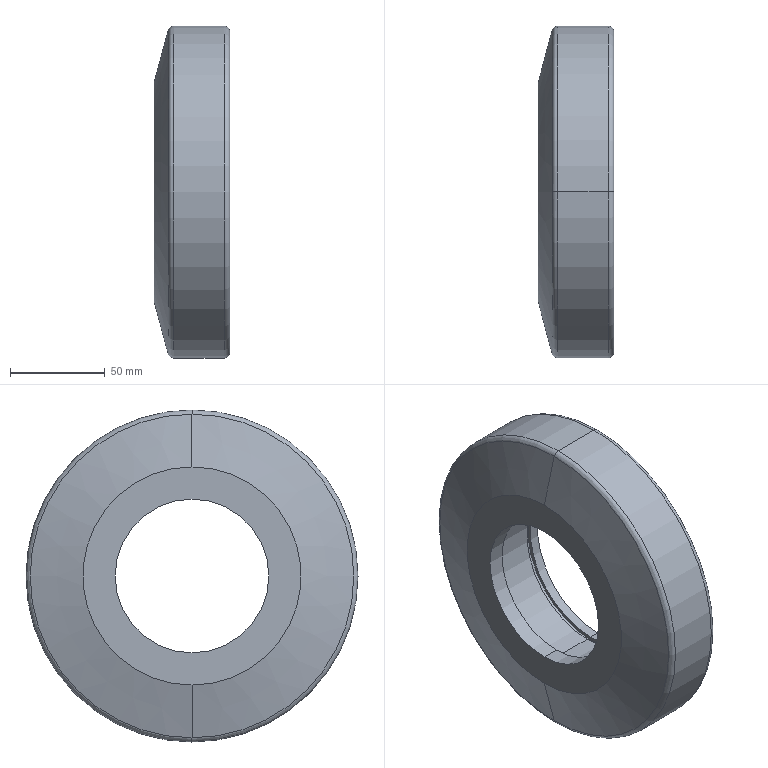Part | STEP file | 02-Guide roller 2 | 1 solid | 21 faces | box 40 x 175 x 175 mm | volume 657116 mm3 | cylinder 10 | plane 5 | torus 4 | cone 2 | commonest cylinder face diameters 90 x4 81 x2 93.5 x2 175 x2
STEP:
#1=CARTESIAN_POINT('',(0.,0.,0.));
#2=DIRECTION('',(0.,0.,1.));
#3=DIRECTION('',(1.,0.,0.));
#4=AXIS2_PLACEMENT_3D('',#1,#2,#3);
#5=CARTESIAN_POINT('',(9.,0.,40.5));
#6=VERTEX_POINT('',#5);
#7=CARTESIAN_POINT('',(0.,0.,40.5));
#8=VERTEX_POINT('',#7);
#9=CARTESIAN_POINT('',(0.,0.,40.5));
#10=DIRECTION('',(-1.,0.,0.));
#11=VECTOR('',#10,1.);
#12=LINE('',#9,#11);
#13=CARTESIAN_POINT('',(0.,0.,0.));
#14=DIRECTION('',(-1.,0.,0.));
#15=DIRECTION('',(0.,0.,1.));
#16=AXIS2_PLACEMENT_3D('',#13,#14,#15);
#17=CYLINDRICAL_SURFACE('',#16,40.5);
#18=CARTESIAN_POINT('',(6.283,0.));
#19=DIRECTION('',(0.,1.));
#20=VECTOR('',#19,1.);
#21=LINE('',#18,#20);
#22=(GEOMETRIC_REPRESENTATION_CONTEXT(2)PARAMETRIC_REPRESENTATION_CONTEXT()REPRESENTATION_CONTEXT('',''));
#23=DEFINITIONAL_REPRESENTATION('',(#21),#22);
#24=PCURVE('',#17,#23);
#25=CARTESIAN_POINT('',(0.,0.,0.));
#26=DIRECTION('',(-1.,0.,0.));
#27=DIRECTION('',(0.,0.,1.));
#28=AXIS2_PLACEMENT_3D('',#25,#26,#27);
#29=CYLINDRICAL_SURFACE('',#28,40.5);
#30=CARTESIAN_POINT('',(0.,0.));
#31=DIRECTION('',(0.,1.));
#32=VECTOR('',#31,1.);
#33=LINE('',#30,#32);
#34=(GEOMETRIC_REPRESENTATION_CONTEXT(2)PARAMETRIC_REPRESENTATION_CONTEXT()REPRESENTATION_CONTEXT('',''));
#35=DEFINITIONAL_REPRESENTATION('',(#33),#34);
#36=PCURVE('',#29,#35);
#37=SURFACE_CURVE('',#12,(#24,#36),.PCURVE_S1.);
#38=EDGE_CURVE('',#6,#8,#37,.T.);
#39=ORIENTED_EDGE('',*,*,#38,.T.);
#40=CARTESIAN_POINT('',(0.,0.,-40.5));
#41=VERTEX_POINT('',#40);
#42=CARTESIAN_POINT('',(0.,0.,0.));
#43=DIRECTION('',(-1.,0.,0.));
#44=DIRECTION('',(0.,0.,1.));
#45=AXIS2_PLACEMENT_3D('',#42,#43,#44);
#46=CIRCLE('',#45,40.5);
#47=CARTESIAN_POINT('',(0.,0.));
#48=DIRECTION('',(1.,0.));
#49=VECTOR('',#48,1.);
#50=LINE('',#47,#49);
#51=(GEOMETRIC_REPRESENTATION_CONTEXT(2)PARAMETRIC_REPRESENTATION_CONTEXT()REPRESENTATION_CONTEXT('',''));
#52=DEFINITIONAL_REPRESENTATION('',(#50),#51);
#53=PCURVE('',#17,#52);
#54=CARTESIAN_POINT('',(0.,40.5,0.));
#55=DIRECTION('',(1.,0.,0.));
#56=DIRECTION('',(0.,0.,-1.));
#57=AXIS2_PLACEMENT_3D('',#54,#55,#56);
#58=PLANE('',#57);
#59=CARTESIAN_POINT('',(-40.5,-40.5));
#60=CARTESIAN_POINT('',(-40.5,29.648));
#61=CARTESIAN_POINT('',(20.25,-5.426));
#62=CARTESIAN_POINT('',(81.,-40.5));
#63=CARTESIAN_POINT('',(20.25,-75.574));
#64=CARTESIAN_POINT('',(-40.5,-110.648));
#65=CARTESIAN_POINT('',(-40.5,-40.5));
#66=(BOUNDED_CURVE()B_SPLINE_CURVE(2,(#59,#60,#61,#62,#63,#64,#65),.UNSPECIFIED.,.T.,.F.)B_SPLINE_CURVE_WITH_KNOTS((1,2,2,2,2,1),(-2.094,0.,2.094,4.189,6.283,8.378),.UNSPECIFIED.)CURVE()GEOMETRIC_REPRESENTATION_ITEM()RATIONAL_B_SPLINE_CURVE((1.,0.5,1.,0.5,1.,0.5,1.))REPRESENTATION_ITEM(''));
#67=(GEOMETRIC_REPRESENTATION_CONTEXT(2)PARAMETRIC_REPRESENTATION_CONTEXT()REPRESENTATION_CONTEXT('',''));
#68=DEFINITIONAL_REPRESENTATION('',(#66),#67);
#69=PCURVE('',#58,#68);
#70=SURFACE_CURVE('',#46,(#53,#69),.PCURVE_S1.);
#71=EDGE_CURVE('',#41,#8,#70,.T.);
#72=ORIENTED_EDGE('',*,*,#71,.F.);
#73=CARTESIAN_POINT('',(9.,0.,-40.5));
#74=VERTEX_POINT('',#73);
#75=CARTESIAN_POINT('',(0.,0.,-40.5));
#76=DIRECTION('',(-1.,0.,0.));
#77=VECTOR('',#76,1.);
#78=LINE('',#75,#77);
#79=CARTESIAN_POINT('',(3.142,0.));
#80=DIRECTION('',(0.,1.));
#81=VECTOR('',#80,1.);
#82=LINE('',#79,#81);
#83=(GEOMETRIC_REPRESENTATION_CONTEXT(2)PARAMETRIC_REPRESENTATION_CONTEXT()REPRESENTATION_CONTEXT('',''));
#84=DEFINITIONAL_REPRESENTATION('',(#82),#83);
#85=PCURVE('',#17,#84);
#86=CARTESIAN_POINT('',(3.142,0.));
#87=DIRECTION('',(0.,1.));
#88=VECTOR('',#87,1.);
#89=LINE('',#86,#88);
#90=(GEOMETRIC_REPRESENTATION_CONTEXT(2)PARAMETRIC_REPRESENTATION_CONTEXT()REPRESENTATION_CONTEXT('',''));
#91=DEFINITIONAL_REPRESENTATION('',(#89),#90);
#92=PCURVE('',#29,#91);
#93=SURFACE_CURVE('',#78,(#85,#92),.PCURVE_S1.);
#94=EDGE_CURVE('',#74,#41,#93,.T.);
#95=ORIENTED_EDGE('',*,*,#94,.F.);
#96=CARTESIAN_POINT('',(9.,0.,0.));
#97=DIRECTION('',(-1.,0.,0.));
#98=DIRECTION('',(0.,0.,1.));
#99=AXIS2_PLACEMENT_3D('',#96,#97,#98);
#100=CIRCLE('',#99,40.5);
#101=CARTESIAN_POINT('',(0.,-9.));
#102=DIRECTION('',(1.,0.));
#103=VECTOR('',#102,1.);
#104=LINE('',#101,#103);
#105=(GEOMETRIC_REPRESENTATION_CONTEXT(2)PARAMETRIC_REPRESENTATION_CONTEXT()REPRESENTATION_CONTEXT('',''));
#106=DEFINITIONAL_REPRESENTATION('',(#104),#105);
#107=PCURVE('',#17,#106);
#108=CARTESIAN_POINT('',(9.,45.,0.));
#109=DIRECTION('',(-1.,0.,0.));
#110=DIRECTION('',(0.,0.,1.));
#111=AXIS2_PLACEMENT_3D('',#108,#109,#110);
#112=PLANE('',#111);
#113=CARTESIAN_POINT('',(0.,-45.));
#114=DIRECTION('',(1.,0.));
#115=AXIS2_PLACEMENT_2D('',#113,#114);
#116=CIRCLE('',#115,40.5);
#117=(GEOMETRIC_REPRESENTATION_CONTEXT(2)PARAMETRIC_REPRESENTATION_CONTEXT()REPRESENTATION_CONTEXT('',''));
#118=DEFINITIONAL_REPRESENTATION('',(#116),#117);
#119=PCURVE('',#112,#118);
#120=SURFACE_CURVE('',#100,(#107,#119),.PCURVE_S1.);
#121=EDGE_CURVE('',#74,#6,#120,.T.);
#122=ORIENTED_EDGE('',*,*,#121,.T.);
#123=EDGE_LOOP('',(#39,#72,#95,#122));
#124=FACE_BOUND('',#123,.F.);
#125=ADVANCED_FACE('',(#124),#17,.F.);
#126=CARTESIAN_POINT('',(32.,0.,45.));
#127=VERTEX_POINT('',#126);
#128=CARTESIAN_POINT('',(9.,0.,45.));
#129=VERTEX_POINT('',#128);
#130=CARTESIAN_POINT('',(0.,0.,45.));
#131=DIRECTION('',(-1.,0.,0.));
#132=VECTOR('',#131,1.);
#133=LINE('',#130,#132);
#134=CARTESIAN_POINT('',(0.,0.,0.));
#135=DIRECTION('',(-1.,0.,0.));
#136=DIRECTION('',(0.,0.,1.));
#137=AXIS2_PLACEMENT_3D('',#134,#135,#136);
#138=CYLINDRICAL_SURFACE('',#137,45.);
#139=CARTESIAN_POINT('',(6.283,0.));
#140=DIRECTION('',(0.,1.));
#141=VECTOR('',#140,1.);
#142=LINE('',#139,#141);
#143=(GEOMETRIC_REPRESENTATION_CONTEXT(2)PARAMETRIC_REPRESENTATION_CONTEXT()REPRESENTATION_CONTEXT('',''));
#144=DEFINITIONAL_REPRESENTATION('',(#142),#143);
#145=PCURVE('',#138,#144);
#146=CARTESIAN_POINT('',(0.,0.,0.));
#147=DIRECTION('',(-1.,0.,0.));
#148=DIRECTION('',(0.,0.,1.));
#149=AXIS2_PLACEMENT_3D('',#146,#147,#148);
#150=CYLINDRICAL_SURFACE('',#149,45.);
#151=CARTESIAN_POINT('',(0.,0.));
#152=DIRECTION('',(0.,1.));
#153=VECTOR('',#152,1.);
#154=LINE('',#151,#153);
#155=(GEOMETRIC_REPRESENTATION_CONTEXT(2)PARAMETRIC_REPRESENTATION_CONTEXT()REPRESENTATION_CONTEXT('',''));
#156=DEFINITIONAL_REPRESENTATION('',(#154),#155);
#157=PCURVE('',#150,#156);
#158=SURFACE_CURVE('',#133,(#145,#157),.PCURVE_S1.);
#159=EDGE_CURVE('',#127,#129,#158,.T.);
#160=ORIENTED_EDGE('',*,*,#159,.T.);
#161=CARTESIAN_POINT('',(9.,0.,-45.));
#162=VERTEX_POINT('',#161);
#163=CARTESIAN_POINT('',(9.,0.,0.));
#164=DIRECTION('',(-1.,0.,0.));
#165=DIRECTION('',(0.,0.,1.));
#166=AXIS2_PLACEMENT_3D('',#163,#164,#165);
#167=CIRCLE('',#166,45.);
#168=CARTESIAN_POINT('',(0.,-9.));
#169=DIRECTION('',(1.,0.));
#170=VECTOR('',#169,1.);
#171=LINE('',#168,#170);
#172=(GEOMETRIC_REPRESENTATION_CONTEXT(2)PARAMETRIC_REPRESENTATION_CONTEXT()REPRESENTATION_CONTEXT('',''));
#173=DEFINITIONAL_REPRESENTATION('',(#171),#172);
#174=PCURVE('',#138,#173);
#175=CARTESIAN_POINT('',(0.,-45.));
#176=DIRECTION('',(1.,0.));
#177=AXIS2_PLACEMENT_2D('',#175,#176);
#178=CIRCLE('',#177,45.);
#179=(GEOMETRIC_REPRESENTATION_CONTEXT(2)PARAMETRIC_REPRESENTATION_CONTEXT()REPRESENTATION_CONTEXT('',''));
#180=DEFINITIONAL_REPRESENTATION('',(#178),#179);
#181=PCURVE('',#112,#180);
#182=SURFACE_CURVE('',#167,(#174,#181),.PCURVE_S1.);
#183=EDGE_CURVE('',#162,#129,#182,.T.);
#184=ORIENTED_EDGE('',*,*,#183,.F.);
#185=CARTESIAN_POINT('',(32.,0.,-45.));
#186=VERTEX_POINT('',#185);
#187=CARTESIAN_POINT('',(0.,0.,-45.));
#188=DIRECTION('',(-1.,0.,0.));
#189=VECTOR('',#188,1.);
#190=LINE('',#187,#189);
#191=CARTESIAN_POINT('',(3.142,0.));
#192=DIRECTION('',(0.,1.));
#193=VECTOR('',#192,1.);
#194=LINE('',#191,#193);
#195=(GEOMETRIC_REPRESENTATION_CONTEXT(2)PARAMETRIC_REPRESENTATION_CONTEXT()REPRESENTATION_CONTEXT('',''));
#196=DEFINITIONAL_REPRESENTATION('',(#194),#195);
#197=PCURVE('',#138,#196);
#198=CARTESIAN_POINT('',(3.142,0.));
#199=DIRECTION('',(0.,1.));
#200=VECTOR('',#199,1.);
#201=LINE('',#198,#200);
#202=(GEOMETRIC_REPRESENTATION_CONTEXT(2)PARAMETRIC_REPRESENTATION_CONTEXT()REPRESENTATION_CONTEXT('',''));
#203=DEFINITIONAL_REPRESENTATION('',(#201),#202);
#204=PCURVE('',#150,#203);
#205=SURFACE_CURVE('',#190,(#197,#204),.PCURVE_S1.);
#206=EDGE_CURVE('',#186,#162,#205,.T.);
#207=ORIENTED_EDGE('',*,*,#206,.F.);
#208=CARTESIAN_POINT('',(32.,0.,0.));
#209=DIRECTION('',(-1.,0.,0.));
#210=DIRECTION('',(0.,0.,1.));
#211=AXIS2_PLACEMENT_3D('',#208,#209,#210);
#212=CIRCLE('',#211,45.);
#213=CARTESIAN_POINT('',(0.,-32.));
#214=DIRECTION('',(1.,0.));
#215=VECTOR('',#214,1.);
#216=LINE('',#213,#215);
#217=(GEOMETRIC_REPRESENTATION_CONTEXT(2)PARAMETRIC_REPRESENTATION_CONTEXT()REPRESENTATION_CONTEXT('',''));
#218=DEFINITIONAL_REPRESENTATION('',(#216),#217);
#219=PCURVE('',#138,#218);
#220=CARTESIAN_POINT('',(32.,46.75,0.));
#221=DIRECTION('',(-1.,0.,0.));
#222=DIRECTION('',(0.,0.,1.));
#223=AXIS2_PLACEMENT_3D('',#220,#221,#222);
#224=PLANE('',#223);
#225=CARTESIAN_POINT('',(0.,-46.75));
#226=DIRECTION('',(1.,0.));
#227=AXIS2_PLACEMENT_2D('',#225,#226);
#228=CIRCLE('',#227,45.);
#229=(GEOMETRIC_REPRESENTATION_CONTEXT(2)PARAMETRIC_REPRESENTATION_CONTEXT()REPRESENTATION_CONTEXT('',''));
#230=DEFINITIONAL_REPRESENTATION('',(#228),#229);
#231=PCURVE('',#224,#230);
#232=SURFACE_CURVE('',#212,(#219,#231),.PCURVE_S1.);
#233=EDGE_CURVE('',#186,#127,#232,.T.);
#234=ORIENTED_EDGE('',*,*,#233,.T.);
#235=EDGE_LOOP('',(#160,#184,#207,#234));
#236=FACE_BOUND('',#235,.F.);
#237=ADVANCED_FACE('',(#236),#138,.F.);
#238=CARTESIAN_POINT('',(34.7,0.,46.75));
#239=VERTEX_POINT('',#238);
#240=CARTESIAN_POINT('',(32.,0.,46.75));
#241=VERTEX_POINT('',#240);
#242=CARTESIAN_POINT('',(0.,0.,46.75));
#243=DIRECTION('',(-1.,0.,0.));
#244=VECTOR('',#243,1.);
#245=LINE('',#242,#244);
#246=CARTESIAN_POINT('',(0.,0.,0.));
#247=DIRECTION('',(-1.,0.,0.));
#248=DIRECTION('',(0.,0.,1.));
#249=AXIS2_PLACEMENT_3D('',#246,#247,#248);
#250=CYLINDRICAL_SURFACE('',#249,46.75);
#251=CARTESIAN_POINT('',(6.283,0.));
#252=DIRECTION('',(0.,1.));
#253=VECTOR('',#252,1.);
#254=LINE('',#251,#253);
#255=(GEOMETRIC_REPRESENTATION_CONTEXT(2)PARAMETRIC_REPRESENTATION_CONTEXT()REPRESENTATION_CONTEXT('',''));
#256=DEFINITIONAL_REPRESENTATION('',(#254),#255);
#257=PCURVE('',#250,#256);
#258=CARTESIAN_POINT('',(0.,0.,0.));
#259=DIRECTION('',(-1.,0.,0.));
#260=DIRECTION('',(0.,0.,1.));
#261=AXIS2_PLACEMENT_3D('',#258,#259,#260);
#262=CYLINDRICAL_SURFACE('',#261,46.75);
#263=CARTESIAN_POINT('',(0.,0.));
#264=DIRECTION('',(0.,1.));
#265=VECTOR('',#264,1.);
#266=LINE('',#263,#265);
#267=(GEOMETRIC_REPRESENTATION_CONTEXT(2)PARAMETRIC_REPRESENTATION_CONTEXT()REPRESENTATION_CONTEXT('',''));
#268=DEFINITIONAL_REPRESENTATION('',(#266),#267);
#269=PCURVE('',#262,#268);
#270=SURFACE_CURVE('',#245,(#257,#269),.PCURVE_S1.);
#271=EDGE_CURVE('',#239,#241,#270,.T.);
#272=ORIENTED_EDGE('',*,*,#271,.T.);
#273=CARTESIAN_POINT('',(32.,0.,-46.75));
#274=VERTEX_POINT('',#273);
#275=CARTESIAN_POINT('',(32.,0.,0.));
#276=DIRECTION('',(-1.,0.,0.));
#277=DIRECTION('',(0.,0.,1.));
#278=AXIS2_PLACEMENT_3D('',#275,#276,#277);
#279=CIRCLE('',#278,46.75);
#280=CARTESIAN_POINT('',(0.,-32.));
#281=DIRECTION('',(1.,0.));
#282=VECTOR('',#281,1.);
#283=LINE('',#280,#282);
#284=(GEOMETRIC_REPRESENTATION_CONTEXT(2)PARAMETRIC_REPRESENTATION_CONTEXT()REPRESENTATION_CONTEXT('',''));
#285=DEFINITIONAL_REPRESENTATION('',(#283),#284);
#286=PCURVE('',#250,#285);
#287=CARTESIAN_POINT('',(0.,-46.75));
#288=DIRECTION('',(1.,0.));
#289=AXIS2_PLACEMENT_2D('',#287,#288);
#290=CIRCLE('',#289,46.75);
#291=(GEOMETRIC_REPRESENTATION_CONTEXT(2)PARAMETRIC_REPRESENTATION_CONTEXT()REPRESENTATION_CONTEXT('',''));
#292=DEFINITIONAL_REPRESENTATION('',(#290),#291);
#293=PCURVE('',#224,#292);
#294=SURFACE_CURVE('',#279,(#286,#293),.PCURVE_S1.);
#295=EDGE_CURVE('',#274,#241,#294,.T.);
#296=ORIENTED_EDGE('',*,*,#295,.F.);
#297=CARTESIAN_POINT('',(34.7,0.,-46.75));
#298=VERTEX_POINT('',#297);
#299=CARTESIAN_POINT('',(0.,0.,-46.75));
#300=DIRECTION('',(-1.,0.,0.));
#301=VECTOR('',#300,1.);
#302=LINE('',#299,#301);
#303=CARTESIAN_POINT('',(3.142,0.));
#304=DIRECTION('',(0.,1.));
#305=VECTOR('',#304,1.);
#306=LINE('',#303,#305);
#307=(GEOMETRIC_REPRESENTATION_CONTEXT(2)PARAMETRIC_REPRESENTATION_CONTEXT()REPRESENTATION_CONTEXT('',''));
#308=DEFINITIONAL_REPRESENTATION('',(#306),#307);
#309=PCURVE('',#250,#308);
#310=CARTESIAN_POINT('',(3.142,0.));
#311=DIRECTION('',(0.,1.));
#312=VECTOR('',#311,1.);
#313=LINE('',#310,#312);
#314=(GEOMETRIC_REPRESENTATION_CONTEXT(2)PARAMETRIC_REPRESENTATION_CONTEXT()REPRESENTATION_CONTEXT('',''));
#315=DEFINITIONAL_REPRESENTATION('',(#313),#314);
#316=PCURVE('',#262,#315);
#317=SURFACE_CURVE('',#302,(#309,#316),.PCURVE_S1.);
#318=EDGE_CURVE('',#298,#274,#317,.T.);
#319=ORIENTED_EDGE('',*,*,#318,.F.);
#320=CARTESIAN_POINT('',(34.7,0.,0.));
#321=DIRECTION('',(-1.,0.,0.));
#322=DIRECTION('',(0.,0.,1.));
#323=AXIS2_PLACEMENT_3D('',#320,#321,#322);
#324=CIRCLE('',#323,46.75);
#325=CARTESIAN_POINT('',(0.,-34.7));
#326=DIRECTION('',(1.,0.));
#327=VECTOR('',#326,1.);
#328=LINE('',#325,#327);
#329=(GEOMETRIC_REPRESENTATION_CONTEXT(2)PARAMETRIC_REPRESENTATION_CONTEXT()REPRESENTATION_CONTEXT('',''));
#330=DEFINITIONAL_REPRESENTATION('',(#328),#329);
#331=PCURVE('',#250,#330);
#332=CARTESIAN_POINT('',(34.7,45.,0.));
#333=DIRECTION('',(1.,0.,0.));
#334=DIRECTION('',(0.,0.,-1.));
#335=AXIS2_PLACEMENT_3D('',#332,#333,#334);
#336=PLANE('',#335);
#337=CARTESIAN_POINT('',(-46.75,-45.));
#338=CARTESIAN_POINT('',(-46.75,35.973));
#339=CARTESIAN_POINT('',(23.375,-4.513));
#340=CARTESIAN_POINT('',(93.5,-45.));
#341=CARTESIAN_POINT('',(23.375,-85.487));
#342=CARTESIAN_POINT('',(-46.75,-125.973));
#343=CARTESIAN_POINT('',(-46.75,-45.));
#344=(BOUNDED_CURVE()B_SPLINE_CURVE(2,(#337,#338,#339,#340,#341,#342,#343),.UNSPECIFIED.,.T.,.F.)B_SPLINE_CURVE_WITH_KNOTS((1,2,2,2,2,1),(-2.094,0.,2.094,4.189,6.283,8.378),.UNSPECIFIED.)CURVE()GEOMETRIC_REPRESENTATION_ITEM()RATIONAL_B_SPLINE_CURVE((1.,0.5,1.,0.5,1.,0.5,1.))REPRESENTATION_ITEM(''));
#345=(GEOMETRIC_REPRESENTATION_CONTEXT(2)PARAMETRIC_REPRESENTATION_CONTEXT()REPRESENTATION_CONTEXT('',''));
#346=DEFINITIONAL_REPRESENTATION('',(#344),#345);
#347=PCURVE('',#336,#346);
#348=SURFACE_CURVE('',#324,(#331,#347),.PCURVE_S1.);
#349=EDGE_CURVE('',#298,#239,#348,.T.);
#350=ORIENTED_EDGE('',*,*,#349,.T.);
#351=EDGE_LOOP('',(#272,#296,#319,#350));
#352=FACE_BOUND('',#351,.F.);
#353=ADVANCED_FACE('',(#352),#250,.F.);
#354=CARTESIAN_POINT('',(40.,0.,45.));
#355=VERTEX_POINT('',#354);
#356=CARTESIAN_POINT('',(34.7,0.,45.));
#357=VERTEX_POINT('',#356);
#358=CARTESIAN_POINT('',(0.,0.,45.));
#359=DIRECTION('',(-1.,0.,0.));
#360=VECTOR('',#359,1.);
#361=LINE('',#358,#360);
#362=CARTESIAN_POINT('',(0.,0.,0.));
#363=DIRECTION('',(-1.,0.,0.));
#364=DIRECTION('',(0.,0.,1.));
#365=AXIS2_PLACEMENT_3D('',#362,#363,#364);
#366=CYLINDRICAL_SURFACE('',#365,45.);
#367=CARTESIAN_POINT('',(6.283,0.));
#368=DIRECTION('',(0.,1.));
#369=VECTOR('',#368,1.);
#370=LINE('',#367,#369);
#371=(GEOMETRIC_REPRESENTATION_CONTEXT(2)PARAMETRIC_REPRESENTATION_CONTEXT()REPRESENTATION_CONTEXT('',''));
#372=DEFINITIONAL_REPRESENTATION('',(#370),#371);
#373=PCURVE('',#366,#372);
#374=CARTESIAN_POINT('',(0.,0.,0.));
#375=DIRECTION('',(-1.,0.,0.));
#376=DIRECTION('',(0.,0.,1.));
#377=AXIS2_PLACEMENT_3D('',#374,#375,#376);
#378=CYLINDRICAL_SURFACE('',#377,45.);
#379=CARTESIAN_POINT('',(0.,0.));
#380=DIRECTION('',(0.,1.));
#381=VECTOR('',#380,1.);
#382=LINE('',#379,#381);
#383=(GEOMETRIC_REPRESENTATION_CONTEXT(2)PARAMETRIC_REPRESENTATION_CONTEXT()REPRESENTATION_CONTEXT('',''));
#384=DEFINITIONAL_REPRESENTATION('',(#382),#383);
#385=PCURVE('',#378,#384);
#386=SURFACE_CURVE('',#361,(#373,#385),.PCURVE_S1.);
#387=EDGE_CURVE('',#355,#357,#386,.T.);
#388=ORIENTED_EDGE('',*,*,#387,.T.);
#389=CARTESIAN_POINT('',(34.7,0.,-45.));
#390=VERTEX_POINT('',#389);
#391=CARTESIAN_POINT('',(34.7,0.,0.));
#392=DIRECTION('',(-1.,0.,0.));
#393=DIRECTION('',(0.,0.,1.));
#394=AXIS2_PLACEMENT_3D('',#391,#392,#393);
#395=CIRCLE('',#394,45.);
#396=CARTESIAN_POINT('',(0.,-34.7));
#397=DIRECTION('',(1.,0.));
#398=VECTOR('',#397,1.);
#399=LINE('',#396,#398);
#400=(GEOMETRIC_REPRESENTATION_CONTEXT(2)PARAMETRIC_REPRESENTATION_CONTEXT()REPRESENTATION_CONTEXT('',''));
#401=DEFINITIONAL_REPRESENTATION('',(#399),#400);
#402=PCURVE('',#366,#401);
#403=CARTESIAN_POINT('',(-45.,-45.));
#404=CARTESIAN_POINT('',(-45.,32.942));
#405=CARTESIAN_POINT('',(22.5,-6.029));
#406=CARTESIAN_POINT('',(90.,-45.));
#407=CARTESIAN_POINT('',(22.5,-83.971));
#408=CARTESIAN_POINT('',(-45.,-122.942));
#409=CARTESIAN_POINT('',(-45.,-45.));
#410=(BOUNDED_CURVE()B_SPLINE_CURVE(2,(#403,#404,#405,#406,#407,#408,#409),.UNSPECIFIED.,.T.,.F.)B_SPLINE_CURVE_WITH_KNOTS((1,2,2,2,2,1),(-2.094,0.,2.094,4.189,6.283,8.378),.UNSPECIFIED.)CURVE()GEOMETRIC_REPRESENTATION_ITEM()RATIONAL_B_SPLINE_CURVE((1.,0.5,1.,0.5,1.,0.5,1.))REPRESENTATION_ITEM(''));
#411=(GEOMETRIC_REPRESENTATION_CONTEXT(2)PARAMETRIC_REPRESENTATION_CONTEXT()REPRESENTATION_CONTEXT('',''));
#412=DEFINITIONAL_REPRESENTATION('',(#410),#411);
#413=PCURVE('',#336,#412);
#414=SURFACE_CURVE('',#395,(#402,#413),.PCURVE_S1.);
#415=EDGE_CURVE('',#390,#357,#414,.T.);
#416=ORIENTED_EDGE('',*,*,#415,.F.);
#417=CARTESIAN_POINT('',(40.,0.,-45.));
#418=VERTEX_POINT('',#417);
#419=CARTESIAN_POINT('',(0.,0.,-45.));
#420=DIRECTION('',(-1.,0.,0.));
#421=VECTOR('',#420,1.);
#422=LINE('',#419,#421);
#423=CARTESIAN_POINT('',(3.142,0.));
#424=DIRECTION('',(0.,1.));
#425=VECTOR('',#424,1.);
#426=LINE('',#423,#425);
#427=(GEOMETRIC_REPRESENTATION_CONTEXT(2)PARAMETRIC_REPRESENTATION_CONTEXT()REPRESENTATION_CONTEXT('',''));
#428=DEFINITIONAL_REPRESENTATION('',(#426),#427);
#429=PCURVE('',#366,#428);
#430=CARTESIAN_POINT('',(3.142,0.));
#431=DIRECTION('',(0.,1.));
#432=VECTOR('',#431,1.);
#433=LINE('',#430,#432);
#434=(GEOMETRIC_REPRESENTATION_CONTEXT(2)PARAMETRIC_REPRESENTATION_CONTEXT()REPRESENTATION_CONTEXT('',''));
#435=DEFINITIONAL_REPRESENTATION('',(#433),#434);
#436=PCURVE('',#378,#435);
#437=SURFACE_CURVE('',#422,(#429,#436),.PCURVE_S1.);
#438=EDGE_CURVE('',#418,#390,#437,.T.);
#439=ORIENTED_EDGE('',*,*,#438,.F.);
#440=CARTESIAN_POINT('',(40.,0.,0.));
#441=DIRECTION('',(-1.,0.,0.));
#442=DIRECTION('',(0.,0.,1.));
#443=AXIS2_PLACEMENT_3D('',#440,#441,#442);
#444=CIRCLE('',#443,45.);
#445=CARTESIAN_POINT('',(0.,-40.));
#446=DIRECTION('',(1.,0.));
#447=VECTOR('',#446,1.);
#448=LINE('',#445,#447);
#449=(GEOMETRIC_REPRESENTATION_CONTEXT(2)PARAMETRIC_REPRESENTATION_CONTEXT()REPRESENTATION_CONTEXT('',''));
#450=DEFINITIONAL_REPRESENTATION('',(#448),#449);
#451=PCURVE('',#366,#450);
#452=CARTESIAN_POINT('',(40.,84.5,0.));
#453=DIRECTION('',(-1.,0.,0.));
#454=DIRECTION('',(0.,0.,1.));
#455=AXIS2_PLACEMENT_3D('',#452,#453,#454);
#456=PLANE('',#455);
#457=CARTESIAN_POINT('',(0.,-84.5));
#458=DIRECTION('',(1.,0.));
#459=AXIS2_PLACEMENT_2D('',#457,#458);
#460=CIRCLE('',#459,45.);
#461=(GEOMETRIC_REPRESENTATION_CONTEXT(2)PARAMETRIC_REPRESENTATION_CONTEXT()REPRESENTATION_CONTEXT('',''));
#462=DEFINITIONAL_REPRESENTATION('',(#460),#461);
#463=PCURVE('',#456,#462);
#464=SURFACE_CURVE('',#444,(#451,#463),.PCURVE_S1.);
#465=EDGE_CURVE('',#418,#355,#464,.T.);
#466=ORIENTED_EDGE('',*,*,#465,.T.);
#467=EDGE_LOOP('',(#388,#416,#439,#466));
#468=FACE_BOUND('',#467,.F.);
#469=ADVANCED_FACE('',(#468),#366,.F.);
#470=CARTESIAN_POINT('',(40.,0.,84.5));
#471=VERTEX_POINT('',#470);
#472=CARTESIAN_POINT('',(40.,0.,-84.5));
#473=VERTEX_POINT('',#472);
#474=CARTESIAN_POINT('',(40.,0.,0.));
#475=DIRECTION('',(-1.,0.,0.));
#476=DIRECTION('',(0.,0.,1.));
#477=AXIS2_PLACEMENT_3D('',#474,#475,#476);
#478=CIRCLE('',#477,84.5);
#479=CARTESIAN_POINT('',(37.,0.,0.));
#480=DIRECTION('',(-1.,0.,0.));
#481=DIRECTION('',(0.,0.,1.));
#482=AXIS2_PLACEMENT_3D('',#479,#480,#481);
#483=TOROIDAL_SURFACE('',#482,84.5,3.);
#484=CARTESIAN_POINT('',(0.,4.712));
#485=DIRECTION('',(1.,0.));
#486=VECTOR('',#485,1.);
#487=LINE('',#484,#486);
#488=(GEOMETRIC_REPRESENTATION_CONTEXT(2)PARAMETRIC_REPRESENTATION_CONTEXT()REPRESENTATION_CONTEXT('',''));
#489=DEFINITIONAL_REPRESENTATION('',(#487),#488);
#490=PCURVE('',#483,#489);
#491=CARTESIAN_POINT('',(0.,-84.5));
#492=DIRECTION('',(1.,0.));
#493=AXIS2_PLACEMENT_2D('',#491,#492);
#494=CIRCLE('',#493,84.5);
#495=(GEOMETRIC_REPRESENTATION_CONTEXT(2)PARAMETRIC_REPRESENTATION_CONTEXT()REPRESENTATION_CONTEXT('',''));
#496=DEFINITIONAL_REPRESENTATION('',(#494),#495);
#497=PCURVE('',#456,#496);
#498=SURFACE_CURVE('',#478,(#490,#497),.PCURVE_S1.);
#499=EDGE_CURVE('',#471,#473,#498,.T.);
#500=ORIENTED_EDGE('',*,*,#499,.T.);
#501=CARTESIAN_POINT('',(37.,0.,-87.5));
#502=VERTEX_POINT('',#501);
#503=CARTESIAN_POINT('',(37.,0.,-84.5));
#504=DIRECTION('',(0.,1.,0.));
#505=DIRECTION('',(0.,0.,1.));
#506=AXIS2_PLACEMENT_3D('',#503,#504,#505);
#507=CIRCLE('',#506,3.);
#508=CARTESIAN_POINT('',(3.142,3.142));
#509=DIRECTION('',(0.,1.));
#510=VECTOR('',#509,1.);
#511=LINE('',#508,#510);
#512=(GEOMETRIC_REPRESENTATION_CONTEXT(2)PARAMETRIC_REPRESENTATION_CONTEXT()REPRESENTATION_CONTEXT('',''));
#513=DEFINITIONAL_REPRESENTATION('',(#511),#512);
#514=PCURVE('',#483,#513);
#515=CARTESIAN_POINT('',(37.,0.,0.));
#516=DIRECTION('',(-1.,0.,0.));
#517=DIRECTION('',(0.,0.,1.));
#518=AXIS2_PLACEMENT_3D('',#515,#516,#517);
#519=TOROIDAL_SURFACE('',#518,84.5,3.);
#520=CARTESIAN_POINT('',(3.142,3.142));
#521=DIRECTION('',(0.,1.));
#522=VECTOR('',#521,1.);
#523=LINE('',#520,#522);
#524=(GEOMETRIC_REPRESENTATION_CONTEXT(2)PARAMETRIC_REPRESENTATION_CONTEXT()REPRESENTATION_CONTEXT('',''));
#525=DEFINITIONAL_REPRESENTATION('',(#523),#524);
#526=PCURVE('',#519,#525);
#527=SURFACE_CURVE('',#507,(#514,#526),.PCURVE_S1.);
#528=EDGE_CURVE('',#473,#502,#527,.T.);
#529=ORIENTED_EDGE('',*,*,#528,.T.);
#530=CARTESIAN_POINT('',(37.,0.,87.5));
#531=VERTEX_POINT('',#530);
#532=CARTESIAN_POINT('',(37.,0.,0.));
#533=DIRECTION('',(-1.,0.,0.));
#534=DIRECTION('',(0.,0.,1.));
#535=AXIS2_PLACEMENT_3D('',#532,#533,#534);
#536=CIRCLE('',#535,87.5);
#537=CARTESIAN_POINT('',(0.,6.283));
#538=DIRECTION('',(1.,0.));
#539=VECTOR('',#538,1.);
#540=LINE('',#537,#539);
#541=(GEOMETRIC_REPRESENTATION_CONTEXT(2)PARAMETRIC_REPRESENTATION_CONTEXT()REPRESENTATION_CONTEXT('',''));
#542=DEFINITIONAL_REPRESENTATION('',(#540),#541);
#543=PCURVE('',#483,#542);
#544=CARTESIAN_POINT('',(0.,0.,0.));
#545=DIRECTION('',(-1.,0.,0.));
#546=DIRECTION('',(0.,0.,1.));
#547=AXIS2_PLACEMENT_3D('',#544,#545,#546);
#548=CYLINDRICAL_SURFACE('',#547,87.5);
#549=CARTESIAN_POINT('',(0.,-37.));
#550=DIRECTION('',(1.,0.));
#551=VECTOR('',#550,1.);
#552=LINE('',#549,#551);
#553=(GEOMETRIC_REPRESENTATION_CONTEXT(2)PARAMETRIC_REPRESENTATION_CONTEXT()REPRESENTATION_CONTEXT('',''));
#554=DEFINITIONAL_REPRESENTATION('',(#552),#553);
#555=PCURVE('',#548,#554);
#556=SURFACE_CURVE('',#536,(#543,#555),.PCURVE_S1.);
#557=EDGE_CURVE('',#531,#502,#556,.T.);
#558=ORIENTED_EDGE('',*,*,#557,.F.);
#559=CARTESIAN_POINT('',(37.,0.,84.5));
#560=DIRECTION('',(0.,-1.,0.));
#561=DIRECTION('',(0.,0.,-1.));
#562=AXIS2_PLACEMENT_3D('',#559,#560,#561);
#563=CIRCLE('',#562,3.);
#564=CARTESIAN_POINT('',(0.,3.142));
#565=DIRECTION('',(0.,1.));
#566=VECTOR('',#565,1.);
#567=LINE('',#564,#566);
#568=(GEOMETRIC_REPRESENTATION_CONTEXT(2)PARAMETRIC_REPRESENTATION_CONTEXT()REPRESENTATION_CONTEXT('',''));
#569=DEFINITIONAL_REPRESENTATION('',(#567),#568);
#570=PCURVE('',#483,#569);
#571=CARTESIAN_POINT('',(6.283,3.142));
#572=DIRECTION('',(0.,1.));
#573=VECTOR('',#572,1.);
#574=LINE('',#571,#573);
#575=(GEOMETRIC_REPRESENTATION_CONTEXT(2)PARAMETRIC_REPRESENTATION_CONTEXT()REPRESENTATION_CONTEXT('',''));
#576=DEFINITIONAL_REPRESENTATION('',(#574),#575);
#577=PCURVE('',#519,#576);
#578=SURFACE_CURVE('',#563,(#570,#577),.PCURVE_S1.);
#579=EDGE_CURVE('',#471,#531,#578,.T.);
#580=ORIENTED_EDGE('',*,*,#579,.F.);
#581=EDGE_LOOP('',(#500,#529,#558,#580));
#582=FACE_BOUND('',#581,.T.);
#583=ADVANCED_FACE('',(#582),#483,.T.);
#584=ORIENTED_EDGE('',*,*,#557,.T.);
#585=CARTESIAN_POINT('',(10.305,0.,-87.5));
#586=VERTEX_POINT('',#585);
#587=CARTESIAN_POINT('',(0.,0.,-87.5));
#588=DIRECTION('',(-1.,0.,0.));
#589=VECTOR('',#588,1.);
#590=LINE('',#587,#589);
#591=CARTESIAN_POINT('',(3.142,0.));
#592=DIRECTION('',(0.,1.));
#593=VECTOR('',#592,1.);
#594=LINE('',#591,#593);
#595=(GEOMETRIC_REPRESENTATION_CONTEXT(2)PARAMETRIC_REPRESENTATION_CONTEXT()REPRESENTATION_CONTEXT('',''));
#596=DEFINITIONAL_REPRESENTATION('',(#594),#595);
#597=PCURVE('',#548,#596);
#598=CARTESIAN_POINT('',(0.,0.,0.));
#599=DIRECTION('',(-1.,0.,0.));
#600=DIRECTION('',(0.,0.,1.));
#601=AXIS2_PLACEMENT_3D('',#598,#599,#600);
#602=CYLINDRICAL_SURFACE('',#601,87.5);
#603=CARTESIAN_POINT('',(3.142,0.));
#604=DIRECTION('',(0.,1.));
#605=VECTOR('',#604,1.);
#606=LINE('',#603,#605);
#607=(GEOMETRIC_REPRESENTATION_CONTEXT(2)PARAMETRIC_REPRESENTATION_CONTEXT()REPRESENTATION_CONTEXT('',''));
#608=DEFINITIONAL_REPRESENTATION('',(#606),#607);
#609=PCURVE('',#602,#608);
#610=SURFACE_CURVE('',#590,(#597,#609),.PCURVE_S1.);
#611=EDGE_CURVE('',#502,#586,#610,.T.);
#612=ORIENTED_EDGE('',*,*,#611,.T.);
#613=CARTESIAN_POINT('',(10.305,0.,87.5));
#614=VERTEX_POINT('',#613);
#615=CARTESIAN_POINT('',(10.305,0.,0.));
#616=DIRECTION('',(-1.,0.,0.));
#617=DIRECTION('',(0.,0.,1.));
#618=AXIS2_PLACEMENT_3D('',#615,#616,#617);
#619=CIRCLE('',#618,87.5);
#620=CARTESIAN_POINT('',(0.,-10.305));
#621=DIRECTION('',(1.,0.));
#622=VECTOR('',#621,1.);
#623=LINE('',#620,#622);
#624=(GEOMETRIC_REPRESENTATION_CONTEXT(2)PARAMETRIC_REPRESENTATION_CONTEXT()REPRESENTATION_CONTEXT('',''));
#625=DEFINITIONAL_REPRESENTATION('',(#623),#624);
#626=PCURVE('',#548,#625);
#627=CARTESIAN_POINT('',(10.305,0.,0.));
#628=DIRECTION('',(-1.,0.,0.));
#629=DIRECTION('',(0.,0.,1.));
#630=AXIS2_PLACEMENT_3D('',#627,#628,#629);
#631=TOROIDAL_SURFACE('',#630,84.5,3.);
#632=CARTESIAN_POINT('',(0.,0.));
#633=DIRECTION('',(1.,0.));
#634=VECTOR('',#633,1.);
#635=LINE('',#632,#634);
#636=(GEOMETRIC_REPRESENTATION_CONTEXT(2)PARAMETRIC_REPRESENTATION_CONTEXT()REPRESENTATION_CONTEXT('',''));
#637=DEFINITIONAL_REPRESENTATION('',(#635),#636);
#638=PCURVE('',#631,#637);
#639=SURFACE_CURVE('',#619,(#626,#638),.PCURVE_S1.);
#640=EDGE_CURVE('',#614,#586,#639,.T.);
#641=ORIENTED_EDGE('',*,*,#640,.F.);
#642=CARTESIAN_POINT('',(0.,0.,87.5));
#643=DIRECTION('',(-1.,0.,0.));
#644=VECTOR('',#643,1.);
#645=LINE('',#642,#644);
#646=CARTESIAN_POINT('',(0.,0.));
#647=DIRECTION('',(0.,1.));
#648=VECTOR('',#647,1.);
#649=LINE('',#646,#648);
#650=(GEOMETRIC_REPRESENTATION_CONTEXT(2)PARAMETRIC_REPRESENTATION_CONTEXT()REPRESENTATION_CONTEXT('',''));
#651=DEFINITIONAL_REPRESENTATION('',(#649),#650);
#652=PCURVE('',#548,#651);
#653=CARTESIAN_POINT('',(6.283,0.));
#654=DIRECTION('',(0.,1.));
#655=VECTOR('',#654,1.);
#656=LINE('',#653,#655);
#657=(GEOMETRIC_REPRESENTATION_CONTEXT(2)PARAMETRIC_REPRESENTATION_CONTEXT()REPRESENTATION_CONTEXT('',''));
#658=DEFINITIONAL_REPRESENTATION('',(#656),#657);
#659=PCURVE('',#602,#658);
#660=SURFACE_CURVE('',#645,(#652,#659),.PCURVE_S1.);
#661=EDGE_CURVE('',#531,#614,#660,.T.);
#662=ORIENTED_EDGE('',*,*,#661,.F.);
#663=EDGE_LOOP('',(#584,#612,#641,#662));
#664=FACE_BOUND('',#663,.T.);
#665=ADVANCED_FACE('',(#664),#548,.T.);
#666=ORIENTED_EDGE('',*,*,#640,.T.);
#667=CARTESIAN_POINT('',(7.406,0.,-85.273));
#668=VERTEX_POINT('',#667);
#669=CARTESIAN_POINT('',(10.305,0.,-84.5));
#670=DIRECTION('',(0.,1.,0.));
#671=DIRECTION('',(0.,0.,1.));
#672=AXIS2_PLACEMENT_3D('',#669,#670,#671);
#673=CIRCLE('',#672,3.);
#674=CARTESIAN_POINT('',(3.142,-3.142));
#675=DIRECTION('',(0.,1.));
#676=VECTOR('',#675,1.);
#677=LINE('',#674,#676);
#678=(GEOMETRIC_REPRESENTATION_CONTEXT(2)PARAMETRIC_REPRESENTATION_CONTEXT()REPRESENTATION_CONTEXT('',''));
#679=DEFINITIONAL_REPRESENTATION('',(#677),#678);
#680=PCURVE('',#631,#679);
#681=CARTESIAN_POINT('',(10.305,0.,0.));
#682=DIRECTION('',(-1.,0.,0.));
#683=DIRECTION('',(0.,0.,1.));
#684=AXIS2_PLACEMENT_3D('',#681,#682,#683);
#685=TOROIDAL_SURFACE('',#684,84.5,3.);
#686=CARTESIAN_POINT('',(3.142,-3.142));
#687=DIRECTION('',(0.,1.));
#688=VECTOR('',#687,1.);
#689=LINE('',#686,#688);
#690=(GEOMETRIC_REPRESENTATION_CONTEXT(2)PARAMETRIC_REPRESENTATION_CONTEXT()REPRESENTATION_CONTEXT('',''));
#691=DEFINITIONAL_REPRESENTATION('',(#689),#690);
#692=PCURVE('',#685,#691);
#693=SURFACE_CURVE('',#673,(#680,#692),.PCURVE_S1.);
#694=EDGE_CURVE('',#586,#668,#693,.T.);
#695=ORIENTED_EDGE('',*,*,#694,.T.);
#696=CARTESIAN_POINT('',(7.406,0.,85.273));
#697=VERTEX_POINT('',#696);
#698=CARTESIAN_POINT('',(7.406,0.,0.));
#699=DIRECTION('',(-1.,0.,0.));
#700=DIRECTION('',(0.,0.,1.));
#701=AXIS2_PLACEMENT_3D('',#698,#699,#700);
#702=CIRCLE('',#701,85.273);
#703=CARTESIAN_POINT('',(0.,1.31));
#704=DIRECTION('',(1.,0.));
#705=VECTOR('',#704,1.);
#706=LINE('',#703,#705);
#707=(GEOMETRIC_REPRESENTATION_CONTEXT(2)PARAMETRIC_REPRESENTATION_CONTEXT()REPRESENTATION_CONTEXT('',''));
#708=DEFINITIONAL_REPRESENTATION('',(#706),#707);
#709=PCURVE('',#631,#708);
#710=CARTESIAN_POINT('',(7.406,0.,0.));
#711=DIRECTION('',(1.,0.,0.));
#712=DIRECTION('',(0.,0.,-1.));
#713=AXIS2_PLACEMENT_3D('',#710,#711,#712);
#714=CONICAL_SURFACE('',#713,85.273,1.31);
#715=CARTESIAN_POINT('',(3.142,0.));
#716=DIRECTION('',(-1.,0.));
#717=VECTOR('',#716,1.);
#718=LINE('',#715,#717);
#719=(GEOMETRIC_REPRESENTATION_CONTEXT(2)PARAMETRIC_REPRESENTATION_CONTEXT()REPRESENTATION_CONTEXT('',''));
#720=DEFINITIONAL_REPRESENTATION('',(#718),#719);
#721=PCURVE('',#714,#720);
#722=SURFACE_CURVE('',#702,(#709,#721),.PCURVE_S1.);
#723=EDGE_CURVE('',#697,#668,#722,.T.);
#724=ORIENTED_EDGE('',*,*,#723,.F.);
#725=CARTESIAN_POINT('',(10.305,0.,84.5));
#726=DIRECTION('',(0.,-1.,0.));
#727=DIRECTION('',(0.,0.,-1.));
#728=AXIS2_PLACEMENT_3D('',#725,#726,#727);
#729=CIRCLE('',#728,3.);
#730=CARTESIAN_POINT('',(0.,-3.142));
#731=DIRECTION('',(0.,1.));
#732=VECTOR('',#731,1.);
#733=LINE('',#730,#732);
#734=(GEOMETRIC_REPRESENTATION_CONTEXT(2)PARAMETRIC_REPRESENTATION_CONTEXT()REPRESENTATION_CONTEXT('',''));
#735=DEFINITIONAL_REPRESENTATION('',(#733),#734);
#736=PCURVE('',#631,#735);
#737=CARTESIAN_POINT('',(6.283,-3.142));
#738=DIRECTION('',(0.,1.));
#739=VECTOR('',#738,1.);
#740=LINE('',#737,#739);
#741=(GEOMETRIC_REPRESENTATION_CONTEXT(2)PARAMETRIC_REPRESENTATION_CONTEXT()REPRESENTATION_CONTEXT('',''));
#742=DEFINITIONAL_REPRESENTATION('',(#740),#741);
#743=PCURVE('',#685,#742);
#744=SURFACE_CURVE('',#729,(#736,#743),.PCURVE_S1.);
#745=EDGE_CURVE('',#614,#697,#744,.T.);
#746=ORIENTED_EDGE('',*,*,#745,.F.);
#747=EDGE_LOOP('',(#666,#695,#724,#746));
#748=FACE_BOUND('',#747,.T.);
#749=ADVANCED_FACE('',(#748),#631,.T.);
#750=CARTESIAN_POINT('',(0.,0.,57.5));
#751=VERTEX_POINT('',#750);
#752=CARTESIAN_POINT('',(0.,0.,-57.5));
#753=VERTEX_POINT('',#752);
#754=CARTESIAN_POINT('',(0.,0.,0.));
#755=DIRECTION('',(-1.,0.,0.));
#756=DIRECTION('',(0.,0.,1.));
#757=AXIS2_PLACEMENT_3D('',#754,#755,#756);
#758=CIRCLE('',#757,57.5);
#759=CARTESIAN_POINT('',(3.142,-7.406));
#760=DIRECTION('',(-1.,0.));
#761=VECTOR('',#760,1.);
#762=LINE('',#759,#761);
#763=(GEOMETRIC_REPRESENTATION_CONTEXT(2)PARAMETRIC_REPRESENTATION_CONTEXT()REPRESENTATION_CONTEXT('',''));
#764=DEFINITIONAL_REPRESENTATION('',(#762),#763);
#765=PCURVE('',#714,#764);
#766=CARTESIAN_POINT('',(-57.5,-40.5));
#767=CARTESIAN_POINT('',(-57.5,59.093));
#768=CARTESIAN_POINT('',(28.75,9.296));
#769=CARTESIAN_POINT('',(115.,-40.5));
#770=CARTESIAN_POINT('',(28.75,-90.296));
#771=CARTESIAN_POINT('',(-57.5,-140.093));
#772=CARTESIAN_POINT('',(-57.5,-40.5));
#773=(BOUNDED_CURVE()B_SPLINE_CURVE(2,(#766,#767,#768,#769,#770,#771,#772),.UNSPECIFIED.,.T.,.F.)B_SPLINE_CURVE_WITH_KNOTS((1,2,2,2,2,1),(-2.094,0.,2.094,4.189,6.283,8.378),.UNSPECIFIED.)CURVE()GEOMETRIC_REPRESENTATION_ITEM()RATIONAL_B_SPLINE_CURVE((1.,0.5,1.,0.5,1.,0.5,1.))REPRESENTATION_ITEM(''));
#774=(GEOMETRIC_REPRESENTATION_CONTEXT(2)PARAMETRIC_REPRESENTATION_CONTEXT()REPRESENTATION_CONTEXT('',''));
#775=DEFINITIONAL_REPRESENTATION('',(#773),#774);
#776=PCURVE('',#58,#775);
#777=SURFACE_CURVE('',#758,(#765,#776),.PCURVE_S1.);
#778=EDGE_CURVE('',#751,#753,#777,.T.);
#779=ORIENTED_EDGE('',*,*,#778,.F.);
#780=CARTESIAN_POINT('',(7.406,0.,85.273));
#781=DIRECTION('',(0.2577,0.,0.9662));
#782=VECTOR('',#781,1.);
#783=LINE('',#780,#782);
#784=CARTESIAN_POINT('',(3.142,0.));
#785=DIRECTION('',(0.,1.));
#786=VECTOR('',#785,1.);
#787=LINE('',#784,#786);
#788=(GEOMETRIC_REPRESENTATION_CONTEXT(2)PARAMETRIC_REPRESENTATION_CONTEXT()REPRESENTATION_CONTEXT('',''));
#789=DEFINITIONAL_REPRESENTATION('',(#787),#788);
#790=PCURVE('',#714,#789);
#791=CARTESIAN_POINT('',(7.406,0.,0.));
#792=DIRECTION('',(1.,0.,0.));
#793=DIRECTION('',(0.,0.,-1.));
#794=AXIS2_PLACEMENT_3D('',#791,#792,#793);
#795=CONICAL_SURFACE('',#794,85.273,1.31);
#796=CARTESIAN_POINT('',(3.142,0.));
#797=DIRECTION('',(0.,1.));
#798=VECTOR('',#797,1.);
#799=LINE('',#796,#798);
#800=(GEOMETRIC_REPRESENTATION_CONTEXT(2)PARAMETRIC_REPRESENTATION_CONTEXT()REPRESENTATION_CONTEXT('',''));
#801=DEFINITIONAL_REPRESENTATION('',(#799),#800);
#802=PCURVE('',#795,#801);
#803=SURFACE_CURVE('',#783,(#790,#802),.PCURVE_S1.);
#804=EDGE_CURVE('',#751,#697,#803,.T.);
#805=ORIENTED_EDGE('',*,*,#804,.T.);
#806=ORIENTED_EDGE('',*,*,#723,.T.);
#807=CARTESIAN_POINT('',(7.406,0.,-85.273));
#808=DIRECTION('',(0.2577,0.,-0.9662));
#809=VECTOR('',#808,1.);
#810=LINE('',#807,#809);
#811=CARTESIAN_POINT('',(0.,0.));
#812=DIRECTION('',(0.,1.));
#813=VECTOR('',#812,1.);
#814=LINE('',#811,#813);
#815=(GEOMETRIC_REPRESENTATION_CONTEXT(2)PARAMETRIC_REPRESENTATION_CONTEXT()REPRESENTATION_CONTEXT('',''));
#816=DEFINITIONAL_REPRESENTATION('',(#814),#815);
#817=PCURVE('',#714,#816);
#818=CARTESIAN_POINT('',(6.283,0.));
#819=DIRECTION('',(0.,1.));
#820=VECTOR('',#819,1.);
#821=LINE('',#818,#820);
#822=(GEOMETRIC_REPRESENTATION_CONTEXT(2)PARAMETRIC_REPRESENTATION_CONTEXT()REPRESENTATION_CONTEXT('',''));
#823=DEFINITIONAL_REPRESENTATION('',(#821),#822);
#824=PCURVE('',#795,#823);
#825=SURFACE_CURVE('',#810,(#817,#824),.PCURVE_S1.);
#826=EDGE_CURVE('',#753,#668,#825,.T.);
#827=ORIENTED_EDGE('',*,*,#826,.F.);
#828=EDGE_LOOP('',(#779,#805,#806,#827));
#829=FACE_BOUND('',#828,.T.);
#830=ADVANCED_FACE('',(#829),#714,.T.);
#831=CARTESIAN_POINT('',(0.,0.,0.));
#832=DIRECTION('',(-1.,0.,0.));
#833=DIRECTION('',(0.,0.,1.));
#834=AXIS2_PLACEMENT_3D('',#831,#832,#833);
#835=CIRCLE('',#834,40.5);
#836=CARTESIAN_POINT('',(-40.5,-40.5));
#837=CARTESIAN_POINT('',(-40.5,29.648));
#838=CARTESIAN_POINT('',(20.25,-5.426));
#839=CARTESIAN_POINT('',(81.,-40.5));
#840=CARTESIAN_POINT('',(20.25,-75.574));
#841=CARTESIAN_POINT('',(-40.5,-110.648));
#842=CARTESIAN_POINT('',(-40.5,-40.5));
#843=(BOUNDED_CURVE()B_SPLINE_CURVE(2,(#836,#837,#838,#839,#840,#841,#842),.UNSPECIFIED.,.T.,.F.)B_SPLINE_CURVE_WITH_KNOTS((1,2,2,2,2,1),(-2.094,0.,2.094,4.189,6.283,8.378),.UNSPECIFIED.)CURVE()GEOMETRIC_REPRESENTATION_ITEM()RATIONAL_B_SPLINE_CURVE((1.,0.5,1.,0.5,1.,0.5,1.))REPRESENTATION_ITEM(''));
#844=(GEOMETRIC_REPRESENTATION_CONTEXT(2)PARAMETRIC_REPRESENTATION_CONTEXT()REPRESENTATION_CONTEXT('',''));
#845=DEFINITIONAL_REPRESENTATION('',(#843),#844);
#846=PCURVE('',#58,#845);
#847=CARTESIAN_POINT('',(0.,0.));
#848=DIRECTION('',(1.,0.));
#849=VECTOR('',#848,1.);
#850=LINE('',#847,#849);
#851=(GEOMETRIC_REPRESENTATION_CONTEXT(2)PARAMETRIC_REPRESENTATION_CONTEXT()REPRESENTATION_CONTEXT('',''));
#852=DEFINITIONAL_REPRESENTATION('',(#850),#851);
#853=PCURVE('',#29,#852);
#854=SURFACE_CURVE('',#835,(#846,#853),.PCURVE_S1.);
#855=EDGE_CURVE('',#8,#41,#854,.T.);
#856=ORIENTED_EDGE('',*,*,#855,.F.);
#857=ORIENTED_EDGE('',*,*,#71,.F.);
#858=EDGE_LOOP('',(#856,#857));
#859=FACE_BOUND('',#858,.T.);
#860=CARTESIAN_POINT('',(0.,0.,0.));
#861=DIRECTION('',(-1.,0.,0.));
#862=DIRECTION('',(0.,0.,1.));
#863=AXIS2_PLACEMENT_3D('',#860,#861,#862);
#864=CIRCLE('',#863,57.5);
#865=CARTESIAN_POINT('',(-57.5,-40.5));
#866=CARTESIAN_POINT('',(-57.5,59.093));
#867=CARTESIAN_POINT('',(28.75,9.296));
#868=CARTESIAN_POINT('',(115.,-40.5));
#869=CARTESIAN_POINT('',(28.75,-90.296));
#870=CARTESIAN_POINT('',(-57.5,-140.093));
#871=CARTESIAN_POINT('',(-57.5,-40.5));
#872=(BOUNDED_CURVE()B_SPLINE_CURVE(2,(#865,#866,#867,#868,#869,#870,#871),.UNSPECIFIED.,.T.,.F.)B_SPLINE_CURVE_WITH_KNOTS((1,2,2,2,2,1),(-2.094,0.,2.094,4.189,6.283,8.378),.UNSPECIFIED.)CURVE()GEOMETRIC_REPRESENTATION_ITEM()RATIONAL_B_SPLINE_CURVE((1.,0.5,1.,0.5,1.,0.5,1.))REPRESENTATION_ITEM(''));
#873=(GEOMETRIC_REPRESENTATION_CONTEXT(2)PARAMETRIC_REPRESENTATION_CONTEXT()REPRESENTATION_CONTEXT('',''));
#874=DEFINITIONAL_REPRESENTATION('',(#872),#873);
#875=PCURVE('',#58,#874);
#876=CARTESIAN_POINT('',(9.425,-7.406));
#877=DIRECTION('',(-1.,0.));
#878=VECTOR('',#877,1.);
#879=LINE('',#876,#878);
#880=(GEOMETRIC_REPRESENTATION_CONTEXT(2)PARAMETRIC_REPRESENTATION_CONTEXT()REPRESENTATION_CONTEXT('',''));
#881=DEFINITIONAL_REPRESENTATION('',(#879),#880);
#882=PCURVE('',#795,#881);
#883=SURFACE_CURVE('',#864,(#875,#882),.PCURVE_S1.);
#884=EDGE_CURVE('',#753,#751,#883,.T.);
#885=ORIENTED_EDGE('',*,*,#884,.T.);
#886=ORIENTED_EDGE('',*,*,#778,.T.);
#887=EDGE_LOOP('',(#885,#886));
#888=FACE_BOUND('',#887,.T.);
#889=ADVANCED_FACE('',(#859,#888),#58,.F.);
#890=ORIENTED_EDGE('',*,*,#804,.F.);
#891=ORIENTED_EDGE('',*,*,#884,.F.);
#892=ORIENTED_EDGE('',*,*,#826,.T.);
#893=CARTESIAN_POINT('',(7.406,0.,0.));
#894=DIRECTION('',(-1.,0.,0.));
#895=DIRECTION('',(0.,0.,1.));
#896=AXIS2_PLACEMENT_3D('',#893,#894,#895);
#897=CIRCLE('',#896,85.273);
#898=CARTESIAN_POINT('',(9.425,0.));
#899=DIRECTION('',(-1.,0.));
#900=VECTOR('',#899,1.);
#901=LINE('',#898,#900);
#902=(GEOMETRIC_REPRESENTATION_CONTEXT(2)PARAMETRIC_REPRESENTATION_CONTEXT()REPRESENTATION_CONTEXT('',''));
#903=DEFINITIONAL_REPRESENTATION('',(#901),#902);
#904=PCURVE('',#795,#903);
#905=CARTESIAN_POINT('',(0.,1.31));
#906=DIRECTION('',(1.,0.));
#907=VECTOR('',#906,1.);
#908=LINE('',#905,#907);
#909=(GEOMETRIC_REPRESENTATION_CONTEXT(2)PARAMETRIC_REPRESENTATION_CONTEXT()REPRESENTATION_CONTEXT('',''));
#910=DEFINITIONAL_REPRESENTATION('',(#908),#909);
#911=PCURVE('',#685,#910);
#912=SURFACE_CURVE('',#897,(#904,#911),.PCURVE_S1.);
#913=EDGE_CURVE('',#668,#697,#912,.T.);
#914=ORIENTED_EDGE('',*,*,#913,.T.);
#915=EDGE_LOOP('',(#890,#891,#892,#914));
#916=FACE_BOUND('',#915,.T.);
#917=ADVANCED_FACE('',(#916),#795,.T.);
#918=ORIENTED_EDGE('',*,*,#694,.F.);
#919=CARTESIAN_POINT('',(10.305,0.,0.));
#920=DIRECTION('',(-1.,0.,0.));
#921=DIRECTION('',(0.,0.,1.));
#922=AXIS2_PLACEMENT_3D('',#919,#920,#921);
#923=CIRCLE('',#922,87.5);
#924=CARTESIAN_POINT('',(0.,0.));
#925=DIRECTION('',(1.,0.));
#926=VECTOR('',#925,1.);
#927=LINE('',#924,#926);
#928=(GEOMETRIC_REPRESENTATION_CONTEXT(2)PARAMETRIC_REPRESENTATION_CONTEXT()REPRESENTATION_CONTEXT('',''));
#929=DEFINITIONAL_REPRESENTATION('',(#927),#928);
#930=PCURVE('',#685,#929);
#931=CARTESIAN_POINT('',(0.,-10.305));
#932=DIRECTION('',(1.,0.));
#933=VECTOR('',#932,1.);
#934=LINE('',#931,#933);
#935=(GEOMETRIC_REPRESENTATION_CONTEXT(2)PARAMETRIC_REPRESENTATION_CONTEXT()REPRESENTATION_CONTEXT('',''));
#936=DEFINITIONAL_REPRESENTATION('',(#934),#935);
#937=PCURVE('',#602,#936);
#938=SURFACE_CURVE('',#923,(#930,#937),.PCURVE_S1.);
#939=EDGE_CURVE('',#586,#614,#938,.T.);
#940=ORIENTED_EDGE('',*,*,#939,.T.);
#941=ORIENTED_EDGE('',*,*,#745,.T.);
#942=ORIENTED_EDGE('',*,*,#913,.F.);
#943=EDGE_LOOP('',(#918,#940,#941,#942));
#944=FACE_BOUND('',#943,.T.);
#945=ADVANCED_FACE('',(#944),#685,.T.);
#946=ORIENTED_EDGE('',*,*,#611,.F.);
#947=CARTESIAN_POINT('',(37.,0.,0.));
#948=DIRECTION('',(-1.,0.,0.));
#949=DIRECTION('',(0.,0.,1.));
#950=AXIS2_PLACEMENT_3D('',#947,#948,#949);
#951=CIRCLE('',#950,87.5);
#952=CARTESIAN_POINT('',(0.,-37.));
#953=DIRECTION('',(1.,0.));
#954=VECTOR('',#953,1.);
#955=LINE('',#952,#954);
#956=(GEOMETRIC_REPRESENTATION_CONTEXT(2)PARAMETRIC_REPRESENTATION_CONTEXT()REPRESENTATION_CONTEXT('',''));
#957=DEFINITIONAL_REPRESENTATION('',(#955),#956);
#958=PCURVE('',#602,#957);
#959=CARTESIAN_POINT('',(0.,6.283));
#960=DIRECTION('',(1.,0.));
#961=VECTOR('',#960,1.);
#962=LINE('',#959,#961);
#963=(GEOMETRIC_REPRESENTATION_CONTEXT(2)PARAMETRIC_REPRESENTATION_CONTEXT()REPRESENTATION_CONTEXT('',''));
#964=DEFINITIONAL_REPRESENTATION('',(#962),#963);
#965=PCURVE('',#519,#964);
#966=SURFACE_CURVE('',#951,(#958,#965),.PCURVE_S1.);
#967=EDGE_CURVE('',#502,#531,#966,.T.);
#968=ORIENTED_EDGE('',*,*,#967,.T.);
#969=ORIENTED_EDGE('',*,*,#661,.T.);
#970=ORIENTED_EDGE('',*,*,#939,.F.);
#971=EDGE_LOOP('',(#946,#968,#969,#970));
#972=FACE_BOUND('',#971,.T.);
#973=ADVANCED_FACE('',(#972),#602,.T.);
#974=ORIENTED_EDGE('',*,*,#528,.F.);
#975=CARTESIAN_POINT('',(40.,0.,0.));
#976=DIRECTION('',(-1.,0.,0.));
#977=DIRECTION('',(0.,0.,1.));
#978=AXIS2_PLACEMENT_3D('',#975,#976,#977);
#979=CIRCLE('',#978,84.5);
#980=CARTESIAN_POINT('',(0.,4.712));
#981=DIRECTION('',(1.,0.));
#982=VECTOR('',#981,1.);
#983=LINE('',#980,#982);
#984=(GEOMETRIC_REPRESENTATION_CONTEXT(2)PARAMETRIC_REPRESENTATION_CONTEXT()REPRESENTATION_CONTEXT('',''));
#985=DEFINITIONAL_REPRESENTATION('',(#983),#984);
#986=PCURVE('',#519,#985);
#987=CARTESIAN_POINT('',(0.,-84.5));
#988=DIRECTION('',(1.,0.));
#989=AXIS2_PLACEMENT_2D('',#987,#988);
#990=CIRCLE('',#989,84.5);
#991=(GEOMETRIC_REPRESENTATION_CONTEXT(2)PARAMETRIC_REPRESENTATION_CONTEXT()REPRESENTATION_CONTEXT('',''));
#992=DEFINITIONAL_REPRESENTATION('',(#990),#991);
#993=PCURVE('',#456,#992);
#994=SURFACE_CURVE('',#979,(#986,#993),.PCURVE_S1.);
#995=EDGE_CURVE('',#473,#471,#994,.T.);
#996=ORIENTED_EDGE('',*,*,#995,.T.);
#997=ORIENTED_EDGE('',*,*,#579,.T.);
#998=ORIENTED_EDGE('',*,*,#967,.F.);
#999=EDGE_LOOP('',(#974,#996,#997,#998));
#1000=FACE_BOUND('',#999,.T.);
#1001=ADVANCED_FACE('',(#1000),#519,.T.);
#1002=ORIENTED_EDGE('',*,*,#499,.F.);
#1003=ORIENTED_EDGE('',*,*,#995,.F.);
#1004=EDGE_LOOP('',(#1002,#1003));
#1005=FACE_BOUND('',#1004,.T.);
#1006=CARTESIAN_POINT('',(40.,0.,0.));
#1007=DIRECTION('',(-1.,0.,0.));
#1008=DIRECTION('',(0.,0.,1.));
#1009=AXIS2_PLACEMENT_3D('',#1006,#1007,#1008);
#1010=CIRCLE('',#1009,45.);
#1011=CARTESIAN_POINT('',(0.,-84.5));
#1012=DIRECTION('',(1.,0.));
#1013=AXIS2_PLACEMENT_2D('',#1011,#1012);
#1014=CIRCLE('',#1013,45.);
#1015=(GEOMETRIC_REPRESENTATION_CONTEXT(2)PARAMETRIC_REPRESENTATION_CONTEXT()REPRESENTATION_CONTEXT('',''));
#1016=DEFINITIONAL_REPRESENTATION('',(#1014),#1015);
#1017=PCURVE('',#456,#1016);
#1018=CARTESIAN_POINT('',(0.,-40.));
#1019=DIRECTION('',(1.,0.));
#1020=VECTOR('',#1019,1.);
#1021=LINE('',#1018,#1020);
#1022=(GEOMETRIC_REPRESENTATION_CONTEXT(2)PARAMETRIC_REPRESENTATION_CONTEXT()REPRESENTATION_CONTEXT('',''));
#1023=DEFINITIONAL_REPRESENTATION('',(#1021),#1022);
#1024=PCURVE('',#378,#1023);
#1025=SURFACE_CURVE('',#1010,(#1017,#1024),.PCURVE_S1.);
#1026=EDGE_CURVE('',#355,#418,#1025,.T.);
#1027=ORIENTED_EDGE('',*,*,#1026,.T.);
#1028=ORIENTED_EDGE('',*,*,#465,.T.);
#1029=EDGE_LOOP('',(#1027,#1028));
#1030=FACE_BOUND('',#1029,.T.);
#1031=ADVANCED_FACE('',(#1005,#1030),#456,.F.);
#1032=CARTESIAN_POINT('',(34.7,0.,0.));
#1033=DIRECTION('',(-1.,0.,0.));
#1034=DIRECTION('',(0.,0.,1.));
#1035=AXIS2_PLACEMENT_3D('',#1032,#1033,#1034);
#1036=CIRCLE('',#1035,45.);
#1037=CARTESIAN_POINT('',(0.,-34.7));
#1038=DIRECTION('',(1.,0.));
#1039=VECTOR('',#1038,1.);
#1040=LINE('',#1037,#1039);
#1041=(GEOMETRIC_REPRESENTATION_CONTEXT(2)PARAMETRIC_REPRESENTATION_CONTEXT()REPRESENTATION_CONTEXT('',''));
#1042=DEFINITIONAL_REPRESENTATION('',(#1040),#1041);
#1043=PCURVE('',#378,#1042);
#1044=CARTESIAN_POINT('',(-45.,-45.));
#1045=CARTESIAN_POINT('',(-45.,32.942));
#1046=CARTESIAN_POINT('',(22.5,-6.029));
#1047=CARTESIAN_POINT('',(90.,-45.));
#1048=CARTESIAN_POINT('',(22.5,-83.971));
#1049=CARTESIAN_POINT('',(-45.,-122.942));
#1050=CARTESIAN_POINT('',(-45.,-45.));
#1051=(BOUNDED_CURVE()B_SPLINE_CURVE(2,(#1044,#1045,#1046,#1047,#1048,#1049,#1050),.UNSPECIFIED.,.T.,.F.)B_SPLINE_CURVE_WITH_KNOTS((1,2,2,2,2,1),(-2.094,0.,2.094,4.189,6.283,8.378),.UNSPECIFIED.)CURVE()GEOMETRIC_REPRESENTATION_ITEM()RATIONAL_B_SPLINE_CURVE((1.,0.5,1.,0.5,1.,0.5,1.))REPRESENTATION_ITEM(''));
#1052=(GEOMETRIC_REPRESENTATION_CONTEXT(2)PARAMETRIC_REPRESENTATION_CONTEXT()REPRESENTATION_CONTEXT('',''));
#1053=DEFINITIONAL_REPRESENTATION('',(#1051),#1052);
#1054=PCURVE('',#336,#1053);
#1055=SURFACE_CURVE('',#1036,(#1043,#1054),.PCURVE_S1.);
#1056=EDGE_CURVE('',#357,#390,#1055,.T.);
#1057=ORIENTED_EDGE('',*,*,#1056,.F.);
#1058=ORIENTED_EDGE('',*,*,#387,.F.);
#1059=ORIENTED_EDGE('',*,*,#1026,.T.);
#1060=ORIENTED_EDGE('',*,*,#438,.T.);
#1061=EDGE_LOOP('',(#1057,#1058,#1059,#1060));
#1062=FACE_BOUND('',#1061,.F.);
#1063=ADVANCED_FACE('',(#1062),#378,.F.);
#1064=ORIENTED_EDGE('',*,*,#1056,.F.);
#1065=ORIENTED_EDGE('',*,*,#415,.F.);
#1066=EDGE_LOOP('',(#1064,#1065));
#1067=FACE_BOUND('',#1066,.T.);
#1068=CARTESIAN_POINT('',(34.7,0.,0.));
#1069=DIRECTION('',(-1.,0.,0.));
#1070=DIRECTION('',(0.,0.,1.));
#1071=AXIS2_PLACEMENT_3D('',#1068,#1069,#1070);
#1072=CIRCLE('',#1071,46.75);
#1073=CARTESIAN_POINT('',(-46.75,-45.));
#1074=CARTESIAN_POINT('',(-46.75,35.973));
#1075=CARTESIAN_POINT('',(23.375,-4.513));
#1076=CARTESIAN_POINT('',(93.5,-45.));
#1077=CARTESIAN_POINT('',(23.375,-85.487));
#1078=CARTESIAN_POINT('',(-46.75,-125.973));
#1079=CARTESIAN_POINT('',(-46.75,-45.));
#1080=(BOUNDED_CURVE()B_SPLINE_CURVE(2,(#1073,#1074,#1075,#1076,#1077,#1078,#1079),.UNSPECIFIED.,.T.,.F.)B_SPLINE_CURVE_WITH_KNOTS((1,2,2,2,2,1),(-2.094,0.,2.094,4.189,6.283,8.378),.UNSPECIFIED.)CURVE()GEOMETRIC_REPRESENTATION_ITEM()RATIONAL_B_SPLINE_CURVE((1.,0.5,1.,0.5,1.,0.5,1.))REPRESENTATION_ITEM(''));
#1081=(GEOMETRIC_REPRESENTATION_CONTEXT(2)PARAMETRIC_REPRESENTATION_CONTEXT()REPRESENTATION_CONTEXT('',''));
#1082=DEFINITIONAL_REPRESENTATION('',(#1080),#1081);
#1083=PCURVE('',#336,#1082);
#1084=CARTESIAN_POINT('',(0.,-34.7));
#1085=DIRECTION('',(1.,0.));
#1086=VECTOR('',#1085,1.);
#1087=LINE('',#1084,#1086);
#1088=(GEOMETRIC_REPRESENTATION_CONTEXT(2)PARAMETRIC_REPRESENTATION_CONTEXT()REPRESENTATION_CONTEXT('',''));
#1089=DEFINITIONAL_REPRESENTATION('',(#1087),#1088);
#1090=PCURVE('',#262,#1089);
#1091=SURFACE_CURVE('',#1072,(#1083,#1090),.PCURVE_S1.);
#1092=EDGE_CURVE('',#239,#298,#1091,.T.);
#1093=ORIENTED_EDGE('',*,*,#1092,.T.);
#1094=ORIENTED_EDGE('',*,*,#349,.T.);
#1095=EDGE_LOOP('',(#1093,#1094));
#1096=FACE_BOUND('',#1095,.T.);
#1097=ADVANCED_FACE('',(#1067,#1096),#336,.F.);
#1098=CARTESIAN_POINT('',(32.,0.,0.));
#1099=DIRECTION('',(-1.,0.,0.));
#1100=DIRECTION('',(0.,0.,1.));
#1101=AXIS2_PLACEMENT_3D('',#1098,#1099,#1100);
#1102=CIRCLE('',#1101,46.75);
#1103=CARTESIAN_POINT('',(0.,-32.));
#1104=DIRECTION('',(1.,0.));
#1105=VECTOR('',#1104,1.);
#1106=LINE('',#1103,#1105);
#1107=(GEOMETRIC_REPRESENTATION_CONTEXT(2)PARAMETRIC_REPRESENTATION_CONTEXT()REPRESENTATION_CONTEXT('',''));
#1108=DEFINITIONAL_REPRESENTATION('',(#1106),#1107);
#1109=PCURVE('',#262,#1108);
#1110=CARTESIAN_POINT('',(0.,-46.75));
#1111=DIRECTION('',(1.,0.));
#1112=AXIS2_PLACEMENT_2D('',#1110,#1111);
#1113=CIRCLE('',#1112,46.75);
#1114=(GEOMETRIC_REPRESENTATION_CONTEXT(2)PARAMETRIC_REPRESENTATION_CONTEXT()REPRESENTATION_CONTEXT('',''));
#1115=DEFINITIONAL_REPRESENTATION('',(#1113),#1114);
#1116=PCURVE('',#224,#1115);
#1117=SURFACE_CURVE('',#1102,(#1109,#1116),.PCURVE_S1.);
#1118=EDGE_CURVE('',#241,#274,#1117,.T.);
#1119=ORIENTED_EDGE('',*,*,#1118,.F.);
#1120=ORIENTED_EDGE('',*,*,#271,.F.);
#1121=ORIENTED_EDGE('',*,*,#1092,.T.);
#1122=ORIENTED_EDGE('',*,*,#318,.T.);
#1123=EDGE_LOOP('',(#1119,#1120,#1121,#1122));
#1124=FACE_BOUND('',#1123,.F.);
#1125=ADVANCED_FACE('',(#1124),#262,.F.);
#1126=ORIENTED_EDGE('',*,*,#1118,.F.);
#1127=ORIENTED_EDGE('',*,*,#295,.F.);
#1128=EDGE_LOOP('',(#1126,#1127));
#1129=FACE_BOUND('',#1128,.T.);
#1130=CARTESIAN_POINT('',(32.,0.,0.));
#1131=DIRECTION('',(-1.,0.,0.));
#1132=DIRECTION('',(0.,0.,1.));
#1133=AXIS2_PLACEMENT_3D('',#1130,#1131,#1132);
#1134=CIRCLE('',#1133,45.);
#1135=CARTESIAN_POINT('',(0.,-46.75));
#1136=DIRECTION('',(1.,0.));
#1137=AXIS2_PLACEMENT_2D('',#1135,#1136);
#1138=CIRCLE('',#1137,45.);
#1139=(GEOMETRIC_REPRESENTATION_CONTEXT(2)PARAMETRIC_REPRESENTATION_CONTEXT()REPRESENTATION_CONTEXT('',''));
#1140=DEFINITIONAL_REPRESENTATION('',(#1138),#1139);
#1141=PCURVE('',#224,#1140);
#1142=CARTESIAN_POINT('',(0.,-32.));
#1143=DIRECTION('',(1.,0.));
#1144=VECTOR('',#1143,1.);
#1145=LINE('',#1142,#1144);
#1146=(GEOMETRIC_REPRESENTATION_CONTEXT(2)PARAMETRIC_REPRESENTATION_CONTEXT()REPRESENTATION_CONTEXT('',''));
#1147=DEFINITIONAL_REPRESENTATION('',(#1145),#1146);
#1148=PCURVE('',#150,#1147);
#1149=SURFACE_CURVE('',#1134,(#1141,#1148),.PCURVE_S1.);
#1150=EDGE_CURVE('',#127,#186,#1149,.T.);
#1151=ORIENTED_EDGE('',*,*,#1150,.T.);
#1152=ORIENTED_EDGE('',*,*,#233,.T.);
#1153=EDGE_LOOP('',(#1151,#1152));
#1154=FACE_BOUND('',#1153,.T.);
#1155=ADVANCED_FACE('',(#1129,#1154),#224,.F.);
#1156=CARTESIAN_POINT('',(9.,0.,0.));
#1157=DIRECTION('',(-1.,0.,0.));
#1158=DIRECTION('',(0.,0.,1.));
#1159=AXIS2_PLACEMENT_3D('',#1156,#1157,#1158);
#1160=CIRCLE('',#1159,45.);
#1161=CARTESIAN_POINT('',(0.,-9.));
#1162=DIRECTION('',(1.,0.));
#1163=VECTOR('',#1162,1.);
#1164=LINE('',#1161,#1163);
#1165=(GEOMETRIC_REPRESENTATION_CONTEXT(2)PARAMETRIC_REPRESENTATION_CONTEXT()REPRESENTATION_CONTEXT('',''));
#1166=DEFINITIONAL_REPRESENTATION('',(#1164),#1165);
#1167=PCURVE('',#150,#1166);
#1168=CARTESIAN_POINT('',(0.,-45.));
#1169=DIRECTION('',(1.,0.));
#1170=AXIS2_PLACEMENT_2D('',#1168,#1169);
#1171=CIRCLE('',#1170,45.);
#1172=(GEOMETRIC_REPRESENTATION_CONTEXT(2)PARAMETRIC_REPRESENTATION_CONTEXT()REPRESENTATION_CONTEXT('',''));
#1173=DEFINITIONAL_REPRESENTATION('',(#1171),#1172);
#1174=PCURVE('',#112,#1173);
#1175=SURFACE_CURVE('',#1160,(#1167,#1174),.PCURVE_S1.);
#1176=EDGE_CURVE('',#129,#162,#1175,.T.);
#1177=ORIENTED_EDGE('',*,*,#1176,.F.);
#1178=ORIENTED_EDGE('',*,*,#159,.F.);
#1179=ORIENTED_EDGE('',*,*,#1150,.T.);
#1180=ORIENTED_EDGE('',*,*,#206,.T.);
#1181=EDGE_LOOP('',(#1177,#1178,#1179,#1180));
#1182=FACE_BOUND('',#1181,.F.);
#1183=ADVANCED_FACE('',(#1182),#150,.F.);
#1184=ORIENTED_EDGE('',*,*,#1176,.F.);
#1185=ORIENTED_EDGE('',*,*,#183,.F.);
#1186=EDGE_LOOP('',(#1184,#1185));
#1187=FACE_BOUND('',#1186,.T.);
#1188=CARTESIAN_POINT('',(9.,0.,0.));
#1189=DIRECTION('',(-1.,0.,0.));
#1190=DIRECTION('',(0.,0.,1.));
#1191=AXIS2_PLACEMENT_3D('',#1188,#1189,#1190);
#1192=CIRCLE('',#1191,40.5);
#1193=CARTESIAN_POINT('',(0.,-45.));
#1194=DIRECTION('',(1.,0.));
#1195=AXIS2_PLACEMENT_2D('',#1193,#1194);
#1196=CIRCLE('',#1195,40.5);
#1197=(GEOMETRIC_REPRESENTATION_CONTEXT(2)PARAMETRIC_REPRESENTATION_CONTEXT()REPRESENTATION_CONTEXT('',''));
#1198=DEFINITIONAL_REPRESENTATION('',(#1196),#1197);
#1199=PCURVE('',#112,#1198);
#1200=CARTESIAN_POINT('',(0.,-9.));
#1201=DIRECTION('',(1.,0.));
#1202=VECTOR('',#1201,1.);
#1203=LINE('',#1200,#1202);
#1204=(GEOMETRIC_REPRESENTATION_CONTEXT(2)PARAMETRIC_REPRESENTATION_CONTEXT()REPRESENTATION_CONTEXT('',''));
#1205=DEFINITIONAL_REPRESENTATION('',(#1203),#1204);
#1206=PCURVE('',#29,#1205);
#1207=SURFACE_CURVE('',#1192,(#1199,#1206),.PCURVE_S1.);
#1208=EDGE_CURVE('',#6,#74,#1207,.T.);
#1209=ORIENTED_EDGE('',*,*,#1208,.T.);
#1210=ORIENTED_EDGE('',*,*,#121,.T.);
#1211=EDGE_LOOP('',(#1209,#1210));
#1212=FACE_BOUND('',#1211,.T.);
#1213=ADVANCED_FACE('',(#1187,#1212),#112,.F.);
#1214=ORIENTED_EDGE('',*,*,#855,.F.);
#1215=ORIENTED_EDGE('',*,*,#38,.F.);
#1216=ORIENTED_EDGE('',*,*,#1208,.T.);
#1217=ORIENTED_EDGE('',*,*,#94,.T.);
#1218=EDGE_LOOP('',(#1214,#1215,#1216,#1217));
#1219=FACE_BOUND('',#1218,.F.);
#1220=ADVANCED_FACE('',(#1219),#29,.F.);
#1221=CLOSED_SHELL('',(#125,#237,#353,#469,#583,#665,#749,#830,#889,#917,#945,#973,#1001,#1031,#1063,#1097,#1125,#1155,#1183,#1213,#1220));
#1222=MANIFOLD_SOLID_BREP('',#1221);
#1223=(LENGTH_UNIT()NAMED_UNIT(*)SI_UNIT(.MILLI.,.METRE.));
#1224=UNCERTAINTY_MEASURE_WITH_UNIT(LENGTH_MEASURE(0.0000001),#1223,'','');
#1225=(NAMED_UNIT(*)PLANE_ANGLE_UNIT()SI_UNIT($,.RADIAN.));
#1226=(NAMED_UNIT(*)SI_UNIT($,.STERADIAN.)SOLID_ANGLE_UNIT());
#1227=(GEOMETRIC_REPRESENTATION_CONTEXT(3)GLOBAL_UNCERTAINTY_ASSIGNED_CONTEXT((#1224))GLOBAL_UNIT_ASSIGNED_CONTEXT((#1223,#1225,#1226))REPRESENTATION_CONTEXT('',''));
#1228=ADVANCED_BREP_SHAPE_REPRESENTATION('',(#4,#1222),#1227);